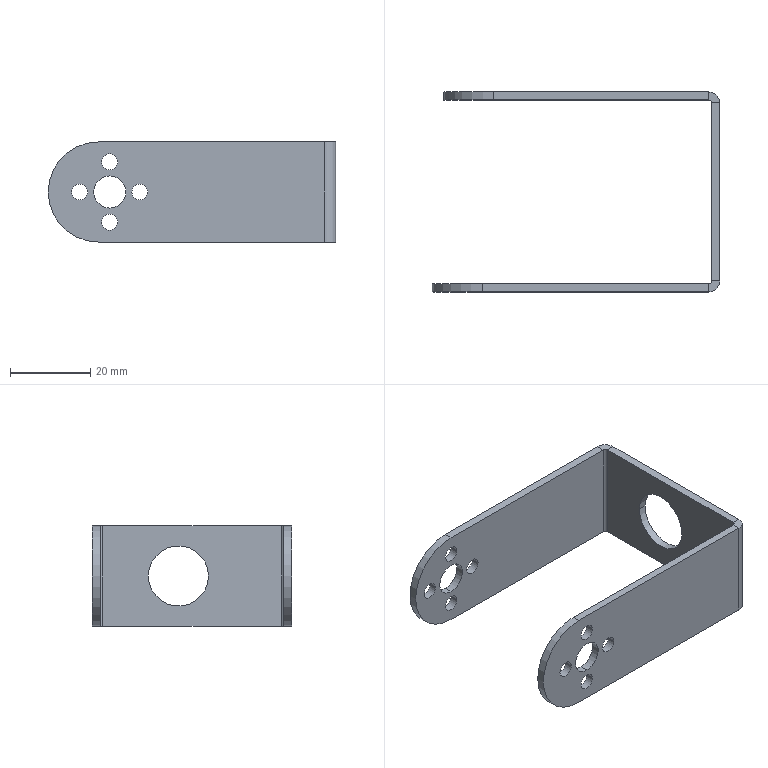Part | SolidWorks | features ICE 3, FlatPattern 1, SM3dBend 1, SMBaseFlange 1, SheetMetal 1 | 1 solid | 44 faces | box 71.712 x 49.895 x 25 mm | volume 8226 mm3 | cylinder 28 | plane 16 | commonest cylinder face diameters 4 x16 8 x4 1.473 x2 5.473 x2 15 x2 25 x2
STEP:
#1=CARTESIAN_POINT('',(-75.172,-2.,-7.5));
#2=VERTEX_POINT('',#1);
#3=CARTESIAN_POINT('',(-79.172,-2.,-7.5));
#4=VERTEX_POINT('',#3);
#5=CARTESIAN_POINT('',(-77.172,-2.,-7.5));
#6=DIRECTION('',(0.,1.,0.));
#7=DIRECTION('',(-1.,0.,0.));
#8=AXIS2_PLACEMENT_3D('',#5,#6,#7);
#9=CIRCLE('',#8,2.);
#10=EDGE_CURVE('',#2,#4,#9,.T.);
#11=ORIENTED_EDGE('',*,*,#10,.F.);
#12=CARTESIAN_POINT('',(-75.172,0.,-7.5));
#13=VERTEX_POINT('',#12);
#14=CARTESIAN_POINT('',(-75.172,-2.,-7.5));
#15=DIRECTION('',(0.,1.,0.));
#16=VECTOR('',#15,1000.);
#17=LINE('',#14,#16);
#18=EDGE_CURVE('',#2,#13,#17,.T.);
#19=ORIENTED_EDGE('',*,*,#18,.T.);
#20=CARTESIAN_POINT('',(-79.172,0.,-7.5));
#21=VERTEX_POINT('',#20);
#22=CARTESIAN_POINT('',(-77.172,0.,-7.5));
#23=DIRECTION('',(0.,1.,0.));
#24=DIRECTION('',(0.,0.,1.));
#25=AXIS2_PLACEMENT_3D('',#22,#23,#24);
#26=CIRCLE('',#25,2.);
#27=EDGE_CURVE('',#13,#21,#26,.T.);
#28=ORIENTED_EDGE('',*,*,#27,.T.);
#29=CARTESIAN_POINT('',(-79.172,-2.,-7.5));
#30=DIRECTION('',(0.,1.,0.));
#31=VECTOR('',#30,1000.);
#32=LINE('',#29,#31);
#33=EDGE_CURVE('',#4,#21,#32,.T.);
#34=ORIENTED_EDGE('',*,*,#33,.F.);
#35=EDGE_LOOP('',(#11,#19,#28,#34));
#36=FACE_OUTER_BOUND('',#35,.T.);
#37=CARTESIAN_POINT('',(-77.172,-2.,-7.5));
#38=DIRECTION('',(0.,1.,0.));
#39=DIRECTION('',(-1.,0.,0.));
#40=AXIS2_PLACEMENT_3D('',#37,#38,#39);
#41=CYLINDRICAL_SURFACE('',#40,2.);
#42=ADVANCED_FACE('',(#36),#41,.F.);
#43=CARTESIAN_POINT('',(-67.672,-2.,0.));
#44=VERTEX_POINT('',#43);
#45=CARTESIAN_POINT('',(-71.672,-2.,0.));
#46=VERTEX_POINT('',#45);
#47=CARTESIAN_POINT('',(-69.672,-2.,0.));
#48=DIRECTION('',(0.,1.,0.));
#49=DIRECTION('',(-1.,0.,0.));
#50=AXIS2_PLACEMENT_3D('',#47,#48,#49);
#51=CIRCLE('',#50,2.);
#52=EDGE_CURVE('',#44,#46,#51,.T.);
#53=ORIENTED_EDGE('',*,*,#52,.F.);
#54=CARTESIAN_POINT('',(-67.672,0.,0.));
#55=VERTEX_POINT('',#54);
#56=CARTESIAN_POINT('',(-67.672,-2.,0.));
#57=DIRECTION('',(0.,1.,0.));
#58=VECTOR('',#57,1000.);
#59=LINE('',#56,#58);
#60=EDGE_CURVE('',#44,#55,#59,.T.);
#61=ORIENTED_EDGE('',*,*,#60,.T.);
#62=CARTESIAN_POINT('',(-71.672,0.,0.));
#63=VERTEX_POINT('',#62);
#64=CARTESIAN_POINT('',(-69.672,0.,0.));
#65=DIRECTION('',(0.,1.,0.));
#66=DIRECTION('',(0.,0.,1.));
#67=AXIS2_PLACEMENT_3D('',#64,#65,#66);
#68=CIRCLE('',#67,2.);
#69=EDGE_CURVE('',#55,#63,#68,.T.);
#70=ORIENTED_EDGE('',*,*,#69,.T.);
#71=CARTESIAN_POINT('',(-71.672,-2.,0.));
#72=DIRECTION('',(0.,1.,0.));
#73=VECTOR('',#72,1000.);
#74=LINE('',#71,#73);
#75=EDGE_CURVE('',#46,#63,#74,.T.);
#76=ORIENTED_EDGE('',*,*,#75,.F.);
#77=EDGE_LOOP('',(#53,#61,#70,#76));
#78=FACE_OUTER_BOUND('',#77,.T.);
#79=CARTESIAN_POINT('',(-69.672,-2.,0.));
#80=DIRECTION('',(0.,1.,0.));
#81=DIRECTION('',(-1.,0.,0.));
#82=AXIS2_PLACEMENT_3D('',#79,#80,#81);
#83=CYLINDRICAL_SURFACE('',#82,2.);
#84=ADVANCED_FACE('',(#78),#83,.F.);
#85=CARTESIAN_POINT('',(-75.172,-2.,7.5));
#86=VERTEX_POINT('',#85);
#87=CARTESIAN_POINT('',(-79.172,-2.,7.5));
#88=VERTEX_POINT('',#87);
#89=CARTESIAN_POINT('',(-77.172,-2.,7.5));
#90=DIRECTION('',(0.,1.,0.));
#91=DIRECTION('',(-1.,0.,0.));
#92=AXIS2_PLACEMENT_3D('',#89,#90,#91);
#93=CIRCLE('',#92,2.);
#94=EDGE_CURVE('',#86,#88,#93,.T.);
#95=ORIENTED_EDGE('',*,*,#94,.F.);
#96=CARTESIAN_POINT('',(-75.172,0.,7.5));
#97=VERTEX_POINT('',#96);
#98=CARTESIAN_POINT('',(-75.172,-2.,7.5));
#99=DIRECTION('',(0.,1.,0.));
#100=VECTOR('',#99,1000.);
#101=LINE('',#98,#100);
#102=EDGE_CURVE('',#86,#97,#101,.T.);
#103=ORIENTED_EDGE('',*,*,#102,.T.);
#104=CARTESIAN_POINT('',(-79.172,0.,7.5));
#105=VERTEX_POINT('',#104);
#106=CARTESIAN_POINT('',(-77.172,0.,7.5));
#107=DIRECTION('',(0.,1.,0.));
#108=DIRECTION('',(0.,0.,1.));
#109=AXIS2_PLACEMENT_3D('',#106,#107,#108);
#110=CIRCLE('',#109,2.);
#111=EDGE_CURVE('',#97,#105,#110,.T.);
#112=ORIENTED_EDGE('',*,*,#111,.T.);
#113=CARTESIAN_POINT('',(-79.172,-2.,7.5));
#114=DIRECTION('',(0.,1.,0.));
#115=VECTOR('',#114,1000.);
#116=LINE('',#113,#115);
#117=EDGE_CURVE('',#88,#105,#116,.T.);
#118=ORIENTED_EDGE('',*,*,#117,.F.);
#119=EDGE_LOOP('',(#95,#103,#112,#118));
#120=FACE_OUTER_BOUND('',#119,.T.);
#121=CARTESIAN_POINT('',(-77.172,-2.,7.5));
#122=DIRECTION('',(0.,1.,0.));
#123=DIRECTION('',(-1.,0.,0.));
#124=AXIS2_PLACEMENT_3D('',#121,#122,#123);
#125=CYLINDRICAL_SURFACE('',#124,2.);
#126=ADVANCED_FACE('',(#120),#125,.F.);
#127=CARTESIAN_POINT('',(-82.672,-2.,0.));
#128=VERTEX_POINT('',#127);
#129=CARTESIAN_POINT('',(-86.672,-2.,0.));
#130=VERTEX_POINT('',#129);
#131=CARTESIAN_POINT('',(-84.672,-2.,0.));
#132=DIRECTION('',(0.,1.,0.));
#133=DIRECTION('',(-1.,0.,0.));
#134=AXIS2_PLACEMENT_3D('',#131,#132,#133);
#135=CIRCLE('',#134,2.);
#136=EDGE_CURVE('',#128,#130,#135,.T.);
#137=ORIENTED_EDGE('',*,*,#136,.F.);
#138=CARTESIAN_POINT('',(-82.672,0.,0.));
#139=VERTEX_POINT('',#138);
#140=CARTESIAN_POINT('',(-82.672,-2.,0.));
#141=DIRECTION('',(0.,1.,0.));
#142=VECTOR('',#141,1000.);
#143=LINE('',#140,#142);
#144=EDGE_CURVE('',#128,#139,#143,.T.);
#145=ORIENTED_EDGE('',*,*,#144,.T.);
#146=CARTESIAN_POINT('',(-86.672,0.,0.));
#147=VERTEX_POINT('',#146);
#148=CARTESIAN_POINT('',(-84.672,0.,0.));
#149=DIRECTION('',(0.,1.,0.));
#150=DIRECTION('',(0.,0.,1.));
#151=AXIS2_PLACEMENT_3D('',#148,#149,#150);
#152=CIRCLE('',#151,2.);
#153=EDGE_CURVE('',#139,#147,#152,.T.);
#154=ORIENTED_EDGE('',*,*,#153,.T.);
#155=CARTESIAN_POINT('',(-86.672,-2.,0.));
#156=DIRECTION('',(0.,1.,0.));
#157=VECTOR('',#156,1000.);
#158=LINE('',#155,#157);
#159=EDGE_CURVE('',#130,#147,#158,.T.);
#160=ORIENTED_EDGE('',*,*,#159,.F.);
#161=EDGE_LOOP('',(#137,#145,#154,#160));
#162=FACE_OUTER_BOUND('',#161,.T.);
#163=CARTESIAN_POINT('',(-84.672,-2.,0.));
#164=DIRECTION('',(0.,1.,0.));
#165=DIRECTION('',(-1.,0.,0.));
#166=AXIS2_PLACEMENT_3D('',#163,#164,#165);
#167=CYLINDRICAL_SURFACE('',#166,2.);
#168=ADVANCED_FACE('',(#162),#167,.F.);
#169=CARTESIAN_POINT('',(-79.172,45.895,-7.5));
#170=VERTEX_POINT('',#169);
#171=CARTESIAN_POINT('',(-75.172,45.895,-7.5));
#172=VERTEX_POINT('',#171);
#173=CARTESIAN_POINT('',(-77.172,45.895,-7.5));
#174=DIRECTION('',(0.,-1.,0.));
#175=DIRECTION('',(1.,0.,0.));
#176=AXIS2_PLACEMENT_3D('',#173,#174,#175);
#177=CIRCLE('',#176,2.);
#178=EDGE_CURVE('',#170,#172,#177,.T.);
#179=ORIENTED_EDGE('',*,*,#178,.T.);
#180=CARTESIAN_POINT('',(-75.172,47.895,-7.5));
#181=VERTEX_POINT('',#180);
#182=CARTESIAN_POINT('',(-75.172,-2.,-7.5));
#183=DIRECTION('',(0.,1.,0.));
#184=VECTOR('',#183,1000.);
#185=LINE('',#182,#184);
#186=EDGE_CURVE('',#172,#181,#185,.T.);
#187=ORIENTED_EDGE('',*,*,#186,.T.);
#188=CARTESIAN_POINT('',(-79.172,47.895,-7.5));
#189=VERTEX_POINT('',#188);
#190=CARTESIAN_POINT('',(-77.172,47.895,-7.5));
#191=DIRECTION('',(0.,-1.,0.));
#192=DIRECTION('',(1.,0.,0.));
#193=AXIS2_PLACEMENT_3D('',#190,#191,#192);
#194=CIRCLE('',#193,2.);
#195=EDGE_CURVE('',#189,#181,#194,.T.);
#196=ORIENTED_EDGE('',*,*,#195,.F.);
#197=CARTESIAN_POINT('',(-79.172,-2.,-7.5));
#198=DIRECTION('',(0.,1.,0.));
#199=VECTOR('',#198,1000.);
#200=LINE('',#197,#199);
#201=EDGE_CURVE('',#170,#189,#200,.T.);
#202=ORIENTED_EDGE('',*,*,#201,.F.);
#203=EDGE_LOOP('',(#179,#187,#196,#202));
#204=FACE_OUTER_BOUND('',#203,.T.);
#205=CARTESIAN_POINT('',(-77.172,-2.,-7.5));
#206=DIRECTION('',(0.,1.,0.));
#207=DIRECTION('',(-1.,0.,0.));
#208=AXIS2_PLACEMENT_3D('',#205,#206,#207);
#209=CYLINDRICAL_SURFACE('',#208,2.);
#210=ADVANCED_FACE('',(#204),#209,.F.);
#211=CARTESIAN_POINT('',(-71.672,45.895,0.));
#212=VERTEX_POINT('',#211);
#213=CARTESIAN_POINT('',(-67.672,45.895,0.));
#214=VERTEX_POINT('',#213);
#215=CARTESIAN_POINT('',(-69.672,45.895,0.));
#216=DIRECTION('',(0.,-1.,0.));
#217=DIRECTION('',(1.,0.,0.));
#218=AXIS2_PLACEMENT_3D('',#215,#216,#217);
#219=CIRCLE('',#218,2.);
#220=EDGE_CURVE('',#212,#214,#219,.T.);
#221=ORIENTED_EDGE('',*,*,#220,.T.);
#222=CARTESIAN_POINT('',(-67.672,47.895,0.));
#223=VERTEX_POINT('',#222);
#224=CARTESIAN_POINT('',(-67.672,-2.,0.));
#225=DIRECTION('',(0.,1.,0.));
#226=VECTOR('',#225,1000.);
#227=LINE('',#224,#226);
#228=EDGE_CURVE('',#214,#223,#227,.T.);
#229=ORIENTED_EDGE('',*,*,#228,.T.);
#230=CARTESIAN_POINT('',(-71.672,47.895,0.));
#231=VERTEX_POINT('',#230);
#232=CARTESIAN_POINT('',(-69.672,47.895,0.));
#233=DIRECTION('',(0.,-1.,0.));
#234=DIRECTION('',(1.,0.,0.));
#235=AXIS2_PLACEMENT_3D('',#232,#233,#234);
#236=CIRCLE('',#235,2.);
#237=EDGE_CURVE('',#231,#223,#236,.T.);
#238=ORIENTED_EDGE('',*,*,#237,.F.);
#239=CARTESIAN_POINT('',(-71.672,-2.,0.));
#240=DIRECTION('',(0.,1.,0.));
#241=VECTOR('',#240,1000.);
#242=LINE('',#239,#241);
#243=EDGE_CURVE('',#212,#231,#242,.T.);
#244=ORIENTED_EDGE('',*,*,#243,.F.);
#245=EDGE_LOOP('',(#221,#229,#238,#244));
#246=FACE_OUTER_BOUND('',#245,.T.);
#247=CARTESIAN_POINT('',(-69.672,-2.,0.));
#248=DIRECTION('',(0.,1.,0.));
#249=DIRECTION('',(-1.,0.,0.));
#250=AXIS2_PLACEMENT_3D('',#247,#248,#249);
#251=CYLINDRICAL_SURFACE('',#250,2.);
#252=ADVANCED_FACE('',(#246),#251,.F.);
#253=CARTESIAN_POINT('',(-79.172,45.895,7.5));
#254=VERTEX_POINT('',#253);
#255=CARTESIAN_POINT('',(-75.172,45.895,7.5));
#256=VERTEX_POINT('',#255);
#257=CARTESIAN_POINT('',(-77.172,45.895,7.5));
#258=DIRECTION('',(0.,-1.,0.));
#259=DIRECTION('',(1.,0.,0.));
#260=AXIS2_PLACEMENT_3D('',#257,#258,#259);
#261=CIRCLE('',#260,2.);
#262=EDGE_CURVE('',#254,#256,#261,.T.);
#263=ORIENTED_EDGE('',*,*,#262,.T.);
#264=CARTESIAN_POINT('',(-75.172,47.895,7.5));
#265=VERTEX_POINT('',#264);
#266=CARTESIAN_POINT('',(-75.172,-2.,7.5));
#267=DIRECTION('',(0.,1.,0.));
#268=VECTOR('',#267,1000.);
#269=LINE('',#266,#268);
#270=EDGE_CURVE('',#256,#265,#269,.T.);
#271=ORIENTED_EDGE('',*,*,#270,.T.);
#272=CARTESIAN_POINT('',(-79.172,47.895,7.5));
#273=VERTEX_POINT('',#272);
#274=CARTESIAN_POINT('',(-77.172,47.895,7.5));
#275=DIRECTION('',(0.,-1.,0.));
#276=DIRECTION('',(1.,0.,0.));
#277=AXIS2_PLACEMENT_3D('',#274,#275,#276);
#278=CIRCLE('',#277,2.);
#279=EDGE_CURVE('',#273,#265,#278,.T.);
#280=ORIENTED_EDGE('',*,*,#279,.F.);
#281=CARTESIAN_POINT('',(-79.172,-2.,7.5));
#282=DIRECTION('',(0.,1.,0.));
#283=VECTOR('',#282,1000.);
#284=LINE('',#281,#283);
#285=EDGE_CURVE('',#254,#273,#284,.T.);
#286=ORIENTED_EDGE('',*,*,#285,.F.);
#287=EDGE_LOOP('',(#263,#271,#280,#286));
#288=FACE_OUTER_BOUND('',#287,.T.);
#289=CARTESIAN_POINT('',(-77.172,-2.,7.5));
#290=DIRECTION('',(0.,1.,0.));
#291=DIRECTION('',(-1.,0.,0.));
#292=AXIS2_PLACEMENT_3D('',#289,#290,#291);
#293=CYLINDRICAL_SURFACE('',#292,2.);
#294=ADVANCED_FACE('',(#288),#293,.F.);
#295=CARTESIAN_POINT('',(-86.672,45.895,0.));
#296=VERTEX_POINT('',#295);
#297=CARTESIAN_POINT('',(-82.672,45.895,0.));
#298=VERTEX_POINT('',#297);
#299=CARTESIAN_POINT('',(-84.672,45.895,0.));
#300=DIRECTION('',(0.,-1.,0.));
#301=DIRECTION('',(1.,0.,0.));
#302=AXIS2_PLACEMENT_3D('',#299,#300,#301);
#303=CIRCLE('',#302,2.);
#304=EDGE_CURVE('',#296,#298,#303,.T.);
#305=ORIENTED_EDGE('',*,*,#304,.T.);
#306=CARTESIAN_POINT('',(-82.672,47.895,0.));
#307=VERTEX_POINT('',#306);
#308=CARTESIAN_POINT('',(-82.672,-2.,0.));
#309=DIRECTION('',(0.,1.,0.));
#310=VECTOR('',#309,1000.);
#311=LINE('',#308,#310);
#312=EDGE_CURVE('',#298,#307,#311,.T.);
#313=ORIENTED_EDGE('',*,*,#312,.T.);
#314=CARTESIAN_POINT('',(-86.672,47.895,0.));
#315=VERTEX_POINT('',#314);
#316=CARTESIAN_POINT('',(-84.672,47.895,0.));
#317=DIRECTION('',(0.,-1.,0.));
#318=DIRECTION('',(1.,0.,0.));
#319=AXIS2_PLACEMENT_3D('',#316,#317,#318);
#320=CIRCLE('',#319,2.);
#321=EDGE_CURVE('',#315,#307,#320,.T.);
#322=ORIENTED_EDGE('',*,*,#321,.F.);
#323=CARTESIAN_POINT('',(-86.672,-2.,0.));
#324=DIRECTION('',(0.,1.,0.));
#325=VECTOR('',#324,1000.);
#326=LINE('',#323,#325);
#327=EDGE_CURVE('',#296,#315,#326,.T.);
#328=ORIENTED_EDGE('',*,*,#327,.F.);
#329=EDGE_LOOP('',(#305,#313,#322,#328));
#330=FACE_OUTER_BOUND('',#329,.T.);
#331=CARTESIAN_POINT('',(-84.672,-2.,0.));
#332=DIRECTION('',(0.,1.,0.));
#333=DIRECTION('',(-1.,0.,0.));
#334=AXIS2_PLACEMENT_3D('',#331,#332,#333);
#335=CYLINDRICAL_SURFACE('',#334,2.);
#336=ADVANCED_FACE('',(#330),#335,.F.);
#337=CARTESIAN_POINT('',(-22.788,33.833,0.));
#338=VERTEX_POINT('',#337);
#339=CARTESIAN_POINT('',(-22.788,18.833,0.));
#340=VERTEX_POINT('',#339);
#341=CARTESIAN_POINT('',(-22.788,26.333,0.));
#342=DIRECTION('',(-1.,0.,0.));
#343=DIRECTION('',(0.,-1.,0.));
#344=AXIS2_PLACEMENT_3D('',#341,#342,#343);
#345=CIRCLE('',#344,7.5);
#346=EDGE_CURVE('',#338,#340,#345,.T.);
#347=ORIENTED_EDGE('',*,*,#346,.T.);
#348=CARTESIAN_POINT('',(-20.788,18.833,0.));
#349=VERTEX_POINT('',#348);
#350=CARTESIAN_POINT('',(-30.788,18.833,0.));
#351=DIRECTION('',(1.,0.,0.));
#352=VECTOR('',#351,1000.);
#353=LINE('',#350,#352);
#354=EDGE_CURVE('',#340,#349,#353,.T.);
#355=ORIENTED_EDGE('',*,*,#354,.T.);
#356=CARTESIAN_POINT('',(-20.788,33.833,0.));
#357=VERTEX_POINT('',#356);
#358=CARTESIAN_POINT('',(-20.788,26.333,0.));
#359=DIRECTION('',(1.,0.,0.));
#360=DIRECTION('',(0.,1.,0.));
#361=AXIS2_PLACEMENT_3D('',#358,#359,#360);
#362=CIRCLE('',#361,7.5);
#363=EDGE_CURVE('',#349,#357,#362,.T.);
#364=ORIENTED_EDGE('',*,*,#363,.T.);
#365=CARTESIAN_POINT('',(-30.788,33.833,0.));
#366=DIRECTION('',(1.,0.,0.));
#367=VECTOR('',#366,1000.);
#368=LINE('',#365,#367);
#369=EDGE_CURVE('',#338,#357,#368,.T.);
#370=ORIENTED_EDGE('',*,*,#369,.F.);
#371=EDGE_LOOP('',(#347,#355,#364,#370));
#372=FACE_OUTER_BOUND('',#371,.T.);
#373=CARTESIAN_POINT('',(-30.788,26.333,0.));
#374=DIRECTION('',(1.,0.,0.));
#375=DIRECTION('',(0.,1.,0.));
#376=AXIS2_PLACEMENT_3D('',#373,#374,#375);
#377=CYLINDRICAL_SURFACE('',#376,7.5);
#378=ADVANCED_FACE('',(#372),#377,.F.);
#379=CARTESIAN_POINT('',(-77.172,-2.,-4.));
#380=VERTEX_POINT('',#379);
#381=CARTESIAN_POINT('',(-77.172,-2.,4.));
#382=VERTEX_POINT('',#381);
#383=CARTESIAN_POINT('',(-77.172,-2.,0.));
#384=DIRECTION('',(0.,1.,0.));
#385=DIRECTION('',(0.,0.,1.));
#386=AXIS2_PLACEMENT_3D('',#383,#384,#385);
#387=CIRCLE('',#386,4.);
#388=EDGE_CURVE('',#380,#382,#387,.T.);
#389=ORIENTED_EDGE('',*,*,#388,.F.);
#390=CARTESIAN_POINT('',(-77.172,0.,-4.));
#391=VERTEX_POINT('',#390);
#392=CARTESIAN_POINT('',(-77.172,-2.,-4.));
#393=DIRECTION('',(0.,1.,0.));
#394=VECTOR('',#393,1000.);
#395=LINE('',#392,#394);
#396=EDGE_CURVE('',#380,#391,#395,.T.);
#397=ORIENTED_EDGE('',*,*,#396,.T.);
#398=CARTESIAN_POINT('',(-77.172,0.,4.));
#399=VERTEX_POINT('',#398);
#400=CARTESIAN_POINT('',(-77.172,0.,0.));
#401=DIRECTION('',(0.,1.,0.));
#402=DIRECTION('',(0.,0.,1.));
#403=AXIS2_PLACEMENT_3D('',#400,#401,#402);
#404=CIRCLE('',#403,4.);
#405=EDGE_CURVE('',#391,#399,#404,.T.);
#406=ORIENTED_EDGE('',*,*,#405,.T.);
#407=CARTESIAN_POINT('',(-77.172,-2.,4.));
#408=DIRECTION('',(0.,1.,0.));
#409=VECTOR('',#408,1000.);
#410=LINE('',#407,#409);
#411=EDGE_CURVE('',#382,#399,#410,.T.);
#412=ORIENTED_EDGE('',*,*,#411,.F.);
#413=EDGE_LOOP('',(#389,#397,#406,#412));
#414=FACE_OUTER_BOUND('',#413,.T.);
#415=CARTESIAN_POINT('',(-77.172,-2.,0.));
#416=DIRECTION('',(0.,1.,0.));
#417=DIRECTION('',(0.,0.,1.));
#418=AXIS2_PLACEMENT_3D('',#415,#416,#417);
#419=CYLINDRICAL_SURFACE('',#418,4.);
#420=ADVANCED_FACE('',(#414),#419,.F.);
#421=CARTESIAN_POINT('',(-77.172,45.895,4.));
#422=VERTEX_POINT('',#421);
#423=CARTESIAN_POINT('',(-77.172,45.895,-4.));
#424=VERTEX_POINT('',#423);
#425=CARTESIAN_POINT('',(-77.172,45.895,0.));
#426=DIRECTION('',(0.,-1.,0.));
#427=DIRECTION('',(1.,0.,0.));
#428=AXIS2_PLACEMENT_3D('',#425,#426,#427);
#429=CIRCLE('',#428,4.);
#430=EDGE_CURVE('',#422,#424,#429,.T.);
#431=ORIENTED_EDGE('',*,*,#430,.T.);
#432=CARTESIAN_POINT('',(-77.172,47.895,-4.));
#433=VERTEX_POINT('',#432);
#434=CARTESIAN_POINT('',(-77.172,-2.,-4.));
#435=DIRECTION('',(0.,1.,0.));
#436=VECTOR('',#435,1000.);
#437=LINE('',#434,#436);
#438=EDGE_CURVE('',#424,#433,#437,.T.);
#439=ORIENTED_EDGE('',*,*,#438,.T.);
#440=CARTESIAN_POINT('',(-77.172,47.895,4.));
#441=VERTEX_POINT('',#440);
#442=CARTESIAN_POINT('',(-77.172,47.895,0.));
#443=DIRECTION('',(0.,1.,0.));
#444=DIRECTION('',(0.,0.,1.));
#445=AXIS2_PLACEMENT_3D('',#442,#443,#444);
#446=CIRCLE('',#445,4.);
#447=EDGE_CURVE('',#433,#441,#446,.T.);
#448=ORIENTED_EDGE('',*,*,#447,.T.);
#449=CARTESIAN_POINT('',(-77.172,-2.,4.));
#450=DIRECTION('',(0.,1.,0.));
#451=VECTOR('',#450,1000.);
#452=LINE('',#449,#451);
#453=EDGE_CURVE('',#422,#441,#452,.T.);
#454=ORIENTED_EDGE('',*,*,#453,.F.);
#455=EDGE_LOOP('',(#431,#439,#448,#454));
#456=FACE_OUTER_BOUND('',#455,.T.);
#457=CARTESIAN_POINT('',(-77.172,-2.,0.));
#458=DIRECTION('',(0.,1.,0.));
#459=DIRECTION('',(0.,0.,1.));
#460=AXIS2_PLACEMENT_3D('',#457,#458,#459);
#461=CYLINDRICAL_SURFACE('',#460,4.);
#462=ADVANCED_FACE('',(#456),#461,.F.);
#463=ORIENTED_EDGE('',*,*,#346,.F.);
#464=CARTESIAN_POINT('',(-22.788,26.333,0.));
#465=DIRECTION('',(-1.,0.,0.));
#466=DIRECTION('',(0.,-1.,0.));
#467=AXIS2_PLACEMENT_3D('',#464,#465,#466);
#468=CIRCLE('',#467,7.5);
#469=EDGE_CURVE('',#340,#338,#468,.T.);
#470=ORIENTED_EDGE('',*,*,#469,.F.);
#471=EDGE_LOOP('',(#463,#470));
#472=FACE_BOUND('',#471,.T.);
#473=CARTESIAN_POINT('',(-22.788,0.7366,12.5));
#474=VERTEX_POINT('',#473);
#475=CARTESIAN_POINT('',(-22.788,45.159,12.5));
#476=VERTEX_POINT('',#475);
#477=CARTESIAN_POINT('',(-22.788,-58.466,12.5));
#478=DIRECTION('',(0.,1.,0.));
#479=VECTOR('',#478,1000.);
#480=LINE('',#477,#479);
#481=EDGE_CURVE('',#474,#476,#480,.T.);
#482=ORIENTED_EDGE('',*,*,#481,.T.);
#483=CARTESIAN_POINT('',(-22.788,45.159,-12.5));
#484=VERTEX_POINT('',#483);
#485=CARTESIAN_POINT('',(-22.788,45.159,0.));
#486=DIRECTION('',(0.,0.,-1.));
#487=VECTOR('',#486,1000.);
#488=LINE('',#485,#487);
#489=EDGE_CURVE('',#476,#484,#488,.T.);
#490=ORIENTED_EDGE('',*,*,#489,.T.);
#491=CARTESIAN_POINT('',(-22.788,0.7366,-12.5));
#492=VERTEX_POINT('',#491);
#493=CARTESIAN_POINT('',(-22.788,-58.466,-12.5));
#494=DIRECTION('',(0.,-1.,0.));
#495=VECTOR('',#494,1000.);
#496=LINE('',#493,#495);
#497=EDGE_CURVE('',#484,#492,#496,.T.);
#498=ORIENTED_EDGE('',*,*,#497,.T.);
#499=CARTESIAN_POINT('',(-22.788,0.7366,0.));
#500=DIRECTION('',(0.,0.,-1.));
#501=VECTOR('',#500,1000.);
#502=LINE('',#499,#501);
#503=EDGE_CURVE('',#474,#492,#502,.T.);
#504=ORIENTED_EDGE('',*,*,#503,.F.);
#505=EDGE_LOOP('',(#482,#490,#498,#504));
#506=FACE_OUTER_BOUND('',#505,.T.);
#507=CARTESIAN_POINT('',(-22.788,-58.466,0.));
#508=DIRECTION('',(-1.,0.,0.));
#509=DIRECTION('',(0.,0.,1.));
#510=AXIS2_PLACEMENT_3D('',#507,#508,#509);
#511=PLANE('',#510);
#512=ADVANCED_FACE('',(#472,#506),#511,.T.);
#513=CARTESIAN_POINT('',(-20.788,0.7366,12.5));
#514=VERTEX_POINT('',#513);
#515=CARTESIAN_POINT('',(-20.788,45.159,12.5));
#516=VERTEX_POINT('',#515);
#517=CARTESIAN_POINT('',(-20.788,-58.466,12.5));
#518=DIRECTION('',(0.,1.,0.));
#519=VECTOR('',#518,1000.);
#520=LINE('',#517,#519);
#521=EDGE_CURVE('',#514,#516,#520,.T.);
#522=ORIENTED_EDGE('',*,*,#521,.T.);
#523=CARTESIAN_POINT('',(-20.788,45.159,12.5));
#524=DIRECTION('',(-1.,0.,0.));
#525=VECTOR('',#524,1000.);
#526=LINE('',#523,#525);
#527=EDGE_CURVE('',#516,#476,#526,.T.);
#528=ORIENTED_EDGE('',*,*,#527,.T.);
#529=ORIENTED_EDGE('',*,*,#481,.F.);
#530=CARTESIAN_POINT('',(-20.788,0.7366,12.5));
#531=DIRECTION('',(-1.,0.,0.));
#532=VECTOR('',#531,1000.);
#533=LINE('',#530,#532);
#534=EDGE_CURVE('',#514,#474,#533,.T.);
#535=ORIENTED_EDGE('',*,*,#534,.F.);
#536=EDGE_LOOP('',(#522,#528,#529,#535));
#537=FACE_OUTER_BOUND('',#536,.T.);
#538=CARTESIAN_POINT('',(-20.788,-58.466,12.5));
#539=DIRECTION('',(0.,0.,1.));
#540=DIRECTION('',(0.,1.,0.));
#541=AXIS2_PLACEMENT_3D('',#538,#539,#540);
#542=PLANE('',#541);
#543=ADVANCED_FACE('',(#537),#542,.T.);
#544=ORIENTED_EDGE('',*,*,#497,.F.);
#545=CARTESIAN_POINT('',(-20.788,45.159,-12.5));
#546=VERTEX_POINT('',#545);
#547=CARTESIAN_POINT('',(-20.788,45.159,-12.5));
#548=DIRECTION('',(1.,0.,0.));
#549=VECTOR('',#548,1000.);
#550=LINE('',#547,#549);
#551=EDGE_CURVE('',#484,#546,#550,.T.);
#552=ORIENTED_EDGE('',*,*,#551,.T.);
#553=CARTESIAN_POINT('',(-20.788,0.7366,-12.5));
#554=VERTEX_POINT('',#553);
#555=CARTESIAN_POINT('',(-20.788,-58.466,-12.5));
#556=DIRECTION('',(0.,-1.,0.));
#557=VECTOR('',#556,1000.);
#558=LINE('',#555,#557);
#559=EDGE_CURVE('',#546,#554,#558,.T.);
#560=ORIENTED_EDGE('',*,*,#559,.T.);
#561=CARTESIAN_POINT('',(-20.788,0.7366,-12.5));
#562=DIRECTION('',(1.,0.,0.));
#563=VECTOR('',#562,1000.);
#564=LINE('',#561,#563);
#565=EDGE_CURVE('',#492,#554,#564,.T.);
#566=ORIENTED_EDGE('',*,*,#565,.F.);
#567=EDGE_LOOP('',(#544,#552,#560,#566));
#568=FACE_OUTER_BOUND('',#567,.T.);
#569=CARTESIAN_POINT('',(-20.788,-58.466,-12.5));
#570=DIRECTION('',(0.,0.,-1.));
#571=DIRECTION('',(0.,-1.,0.));
#572=AXIS2_PLACEMENT_3D('',#569,#570,#571);
#573=PLANE('',#572);
#574=ADVANCED_FACE('',(#568),#573,.T.);
#575=CARTESIAN_POINT('',(-20.788,26.333,0.));
#576=DIRECTION('',(1.,0.,0.));
#577=DIRECTION('',(0.,1.,0.));
#578=AXIS2_PLACEMENT_3D('',#575,#576,#577);
#579=CIRCLE('',#578,7.5);
#580=EDGE_CURVE('',#357,#349,#579,.T.);
#581=ORIENTED_EDGE('',*,*,#580,.F.);
#582=ORIENTED_EDGE('',*,*,#363,.F.);
#583=EDGE_LOOP('',(#581,#582));
#584=FACE_BOUND('',#583,.T.);
#585=CARTESIAN_POINT('',(-20.788,45.159,0.));
#586=DIRECTION('',(0.,0.,-1.));
#587=VECTOR('',#586,1000.);
#588=LINE('',#585,#587);
#589=EDGE_CURVE('',#516,#546,#588,.T.);
#590=ORIENTED_EDGE('',*,*,#589,.F.);
#591=ORIENTED_EDGE('',*,*,#521,.F.);
#592=CARTESIAN_POINT('',(-20.788,0.7366,0.));
#593=DIRECTION('',(0.,0.,-1.));
#594=VECTOR('',#593,1000.);
#595=LINE('',#592,#594);
#596=EDGE_CURVE('',#514,#554,#595,.T.);
#597=ORIENTED_EDGE('',*,*,#596,.T.);
#598=ORIENTED_EDGE('',*,*,#559,.F.);
#599=EDGE_LOOP('',(#590,#591,#597,#598));
#600=FACE_OUTER_BOUND('',#599,.T.);
#601=CARTESIAN_POINT('',(-20.788,-58.466,0.));
#602=DIRECTION('',(-1.,0.,0.));
#603=DIRECTION('',(0.,0.,1.));
#604=AXIS2_PLACEMENT_3D('',#601,#602,#603);
#605=PLANE('',#604);
#606=ADVANCED_FACE('',(#584,#600),#605,.F.);
#607=CARTESIAN_POINT('',(-80.,0.,-12.5));
#608=VERTEX_POINT('',#607);
#609=CARTESIAN_POINT('',(-80.,0.,12.5));
#610=VERTEX_POINT('',#609);
#611=CARTESIAN_POINT('',(-80.,0.,0.));
#612=DIRECTION('',(0.,1.,0.));
#613=DIRECTION('',(0.,0.,1.));
#614=AXIS2_PLACEMENT_3D('',#611,#612,#613);
#615=CIRCLE('',#614,12.5);
#616=EDGE_CURVE('',#608,#610,#615,.T.);
#617=ORIENTED_EDGE('',*,*,#616,.F.);
#618=CARTESIAN_POINT('',(-80.,-2.,-12.5));
#619=VERTEX_POINT('',#618);
#620=CARTESIAN_POINT('',(-80.,-2.,-12.5));
#621=DIRECTION('',(0.,1.,0.));
#622=VECTOR('',#621,1000.);
#623=LINE('',#620,#622);
#624=EDGE_CURVE('',#619,#608,#623,.T.);
#625=ORIENTED_EDGE('',*,*,#624,.F.);
#626=CARTESIAN_POINT('',(-80.,-2.,12.5));
#627=VERTEX_POINT('',#626);
#628=CARTESIAN_POINT('',(-80.,-2.,0.));
#629=DIRECTION('',(0.,1.,0.));
#630=DIRECTION('',(0.,0.,1.));
#631=AXIS2_PLACEMENT_3D('',#628,#629,#630);
#632=CIRCLE('',#631,12.5);
#633=EDGE_CURVE('',#619,#627,#632,.T.);
#634=ORIENTED_EDGE('',*,*,#633,.T.);
#635=CARTESIAN_POINT('',(-80.,-2.,12.5));
#636=DIRECTION('',(0.,1.,0.));
#637=VECTOR('',#636,1000.);
#638=LINE('',#635,#637);
#639=EDGE_CURVE('',#627,#610,#638,.T.);
#640=ORIENTED_EDGE('',*,*,#639,.T.);
#641=EDGE_LOOP('',(#617,#625,#634,#640));
#642=FACE_OUTER_BOUND('',#641,.T.);
#643=CARTESIAN_POINT('',(-80.,-2.,0.));
#644=DIRECTION('',(0.,1.,0.));
#645=DIRECTION('',(0.,0.,1.));
#646=AXIS2_PLACEMENT_3D('',#643,#644,#645);
#647=CYLINDRICAL_SURFACE('',#646,12.5);
#648=ADVANCED_FACE('',(#642),#647,.T.);
#649=CARTESIAN_POINT('',(-77.172,-2.,-7.5));
#650=DIRECTION('',(0.,1.,0.));
#651=DIRECTION('',(-1.,0.,0.));
#652=AXIS2_PLACEMENT_3D('',#649,#650,#651);
#653=CIRCLE('',#652,2.);
#654=EDGE_CURVE('',#4,#2,#653,.T.);
#655=ORIENTED_EDGE('',*,*,#654,.T.);
#656=ORIENTED_EDGE('',*,*,#10,.T.);
#657=EDGE_LOOP('',(#655,#656));
#658=FACE_BOUND('',#657,.T.);
#659=CARTESIAN_POINT('',(-69.672,-2.,0.));
#660=DIRECTION('',(0.,1.,0.));
#661=DIRECTION('',(-1.,0.,0.));
#662=AXIS2_PLACEMENT_3D('',#659,#660,#661);
#663=CIRCLE('',#662,2.);
#664=EDGE_CURVE('',#46,#44,#663,.T.);
#665=ORIENTED_EDGE('',*,*,#664,.T.);
#666=ORIENTED_EDGE('',*,*,#52,.T.);
#667=EDGE_LOOP('',(#665,#666));
#668=FACE_BOUND('',#667,.T.);
#669=CARTESIAN_POINT('',(-77.172,-2.,7.5));
#670=DIRECTION('',(0.,1.,0.));
#671=DIRECTION('',(-1.,0.,0.));
#672=AXIS2_PLACEMENT_3D('',#669,#670,#671);
#673=CIRCLE('',#672,2.);
#674=EDGE_CURVE('',#88,#86,#673,.T.);
#675=ORIENTED_EDGE('',*,*,#674,.T.);
#676=ORIENTED_EDGE('',*,*,#94,.T.);
#677=EDGE_LOOP('',(#675,#676));
#678=FACE_BOUND('',#677,.T.);
#679=CARTESIAN_POINT('',(-84.672,-2.,0.));
#680=DIRECTION('',(0.,1.,0.));
#681=DIRECTION('',(-1.,0.,0.));
#682=AXIS2_PLACEMENT_3D('',#679,#680,#681);
#683=CIRCLE('',#682,2.);
#684=EDGE_CURVE('',#130,#128,#683,.T.);
#685=ORIENTED_EDGE('',*,*,#684,.T.);
#686=ORIENTED_EDGE('',*,*,#136,.T.);
#687=EDGE_LOOP('',(#685,#686));
#688=FACE_BOUND('',#687,.T.);
#689=CARTESIAN_POINT('',(-77.172,-2.,0.));
#690=DIRECTION('',(0.,1.,0.));
#691=DIRECTION('',(0.,0.,1.));
#692=AXIS2_PLACEMENT_3D('',#689,#690,#691);
#693=CIRCLE('',#692,4.);
#694=EDGE_CURVE('',#382,#380,#693,.T.);
#695=ORIENTED_EDGE('',*,*,#694,.T.);
#696=ORIENTED_EDGE('',*,*,#388,.T.);
#697=EDGE_LOOP('',(#695,#696));
#698=FACE_BOUND('',#697,.T.);
#699=CARTESIAN_POINT('',(-23.525,-2.,12.5));
#700=VERTEX_POINT('',#699);
#701=CARTESIAN_POINT('',(-23.525,-2.,-12.5));
#702=VERTEX_POINT('',#701);
#703=CARTESIAN_POINT('',(-23.525,-2.,0.));
#704=DIRECTION('',(0.,0.,-1.));
#705=VECTOR('',#704,1000.);
#706=LINE('',#703,#705);
#707=EDGE_CURVE('',#700,#702,#706,.T.);
#708=ORIENTED_EDGE('',*,*,#707,.F.);
#709=CARTESIAN_POINT('',(-80.,-2.,12.5));
#710=DIRECTION('',(1.,0.,0.));
#711=VECTOR('',#710,1000.);
#712=LINE('',#709,#711);
#713=EDGE_CURVE('',#627,#700,#712,.T.);
#714=ORIENTED_EDGE('',*,*,#713,.F.);
#715=ORIENTED_EDGE('',*,*,#633,.F.);
#716=CARTESIAN_POINT('',(-80.,-2.,-12.5));
#717=DIRECTION('',(-1.,0.,0.));
#718=VECTOR('',#717,1000.);
#719=LINE('',#716,#718);
#720=EDGE_CURVE('',#702,#619,#719,.T.);
#721=ORIENTED_EDGE('',*,*,#720,.F.);
#722=EDGE_LOOP('',(#708,#714,#715,#721));
#723=FACE_OUTER_BOUND('',#722,.T.);
#724=CARTESIAN_POINT('',(-80.,-2.,0.));
#725=DIRECTION('',(0.,1.,0.));
#726=DIRECTION('',(0.,0.,1.));
#727=AXIS2_PLACEMENT_3D('',#724,#725,#726);
#728=PLANE('',#727);
#729=ADVANCED_FACE('',(#658,#668,#678,#688,#698,#723),#728,.F.);
#730=ORIENTED_EDGE('',*,*,#713,.T.);
#731=CARTESIAN_POINT('',(-23.525,0.,12.5));
#732=VERTEX_POINT('',#731);
#733=CARTESIAN_POINT('',(-23.525,-2.,12.5));
#734=DIRECTION('',(0.,1.,0.));
#735=VECTOR('',#734,1000.);
#736=LINE('',#733,#735);
#737=EDGE_CURVE('',#700,#732,#736,.T.);
#738=ORIENTED_EDGE('',*,*,#737,.T.);
#739=CARTESIAN_POINT('',(-80.,0.,12.5));
#740=DIRECTION('',(1.,0.,0.));
#741=VECTOR('',#740,1000.);
#742=LINE('',#739,#741);
#743=EDGE_CURVE('',#610,#732,#742,.T.);
#744=ORIENTED_EDGE('',*,*,#743,.F.);
#745=ORIENTED_EDGE('',*,*,#639,.F.);
#746=EDGE_LOOP('',(#730,#738,#744,#745));
#747=FACE_OUTER_BOUND('',#746,.T.);
#748=CARTESIAN_POINT('',(-80.,-2.,12.5));
#749=DIRECTION('',(0.,0.,1.));
#750=DIRECTION('',(1.,0.,0.));
#751=AXIS2_PLACEMENT_3D('',#748,#749,#750);
#752=PLANE('',#751);
#753=ADVANCED_FACE('',(#747),#752,.T.);
#754=CARTESIAN_POINT('',(-77.172,0.,-7.5));
#755=DIRECTION('',(0.,1.,0.));
#756=DIRECTION('',(0.,0.,1.));
#757=AXIS2_PLACEMENT_3D('',#754,#755,#756);
#758=CIRCLE('',#757,2.);
#759=EDGE_CURVE('',#21,#13,#758,.T.);
#760=ORIENTED_EDGE('',*,*,#759,.F.);
#761=ORIENTED_EDGE('',*,*,#27,.F.);
#762=EDGE_LOOP('',(#760,#761));
#763=FACE_BOUND('',#762,.T.);
#764=CARTESIAN_POINT('',(-69.672,0.,0.));
#765=DIRECTION('',(0.,1.,0.));
#766=DIRECTION('',(0.,0.,1.));
#767=AXIS2_PLACEMENT_3D('',#764,#765,#766);
#768=CIRCLE('',#767,2.);
#769=EDGE_CURVE('',#63,#55,#768,.T.);
#770=ORIENTED_EDGE('',*,*,#769,.F.);
#771=ORIENTED_EDGE('',*,*,#69,.F.);
#772=EDGE_LOOP('',(#770,#771));
#773=FACE_BOUND('',#772,.T.);
#774=CARTESIAN_POINT('',(-77.172,0.,7.5));
#775=DIRECTION('',(0.,1.,0.));
#776=DIRECTION('',(0.,0.,1.));
#777=AXIS2_PLACEMENT_3D('',#774,#775,#776);
#778=CIRCLE('',#777,2.);
#779=EDGE_CURVE('',#105,#97,#778,.T.);
#780=ORIENTED_EDGE('',*,*,#779,.F.);
#781=ORIENTED_EDGE('',*,*,#111,.F.);
#782=EDGE_LOOP('',(#780,#781));
#783=FACE_BOUND('',#782,.T.);
#784=CARTESIAN_POINT('',(-84.672,0.,0.));
#785=DIRECTION('',(0.,1.,0.));
#786=DIRECTION('',(0.,0.,1.));
#787=AXIS2_PLACEMENT_3D('',#784,#785,#786);
#788=CIRCLE('',#787,2.);
#789=EDGE_CURVE('',#147,#139,#788,.T.);
#790=ORIENTED_EDGE('',*,*,#789,.F.);
#791=ORIENTED_EDGE('',*,*,#153,.F.);
#792=EDGE_LOOP('',(#790,#791));
#793=FACE_BOUND('',#792,.T.);
#794=CARTESIAN_POINT('',(-77.172,0.,0.));
#795=DIRECTION('',(0.,1.,0.));
#796=DIRECTION('',(0.,0.,1.));
#797=AXIS2_PLACEMENT_3D('',#794,#795,#796);
#798=CIRCLE('',#797,4.);
#799=EDGE_CURVE('',#399,#391,#798,.T.);
#800=ORIENTED_EDGE('',*,*,#799,.F.);
#801=ORIENTED_EDGE('',*,*,#405,.F.);
#802=EDGE_LOOP('',(#800,#801));
#803=FACE_BOUND('',#802,.T.);
#804=ORIENTED_EDGE('',*,*,#743,.T.);
#805=CARTESIAN_POINT('',(-23.525,0.,-12.5));
#806=VERTEX_POINT('',#805);
#807=CARTESIAN_POINT('',(-23.525,0.,0.));
#808=DIRECTION('',(0.,0.,-1.));
#809=VECTOR('',#808,1000.);
#810=LINE('',#807,#809);
#811=EDGE_CURVE('',#732,#806,#810,.T.);
#812=ORIENTED_EDGE('',*,*,#811,.T.);
#813=CARTESIAN_POINT('',(-80.,0.,-12.5));
#814=DIRECTION('',(-1.,0.,0.));
#815=VECTOR('',#814,1000.);
#816=LINE('',#813,#815);
#817=EDGE_CURVE('',#806,#608,#816,.T.);
#818=ORIENTED_EDGE('',*,*,#817,.T.);
#819=ORIENTED_EDGE('',*,*,#616,.T.);
#820=EDGE_LOOP('',(#804,#812,#818,#819));
#821=FACE_OUTER_BOUND('',#820,.T.);
#822=CARTESIAN_POINT('',(-80.,0.,0.));
#823=DIRECTION('',(0.,1.,0.));
#824=DIRECTION('',(0.,0.,1.));
#825=AXIS2_PLACEMENT_3D('',#822,#823,#824);
#826=PLANE('',#825);
#827=ADVANCED_FACE('',(#763,#773,#783,#793,#803,#821),#826,.T.);
#828=ORIENTED_EDGE('',*,*,#817,.F.);
#829=CARTESIAN_POINT('',(-23.525,-2.,-12.5));
#830=DIRECTION('',(0.,-1.,0.));
#831=VECTOR('',#830,1000.);
#832=LINE('',#829,#831);
#833=EDGE_CURVE('',#806,#702,#832,.T.);
#834=ORIENTED_EDGE('',*,*,#833,.T.);
#835=ORIENTED_EDGE('',*,*,#720,.T.);
#836=ORIENTED_EDGE('',*,*,#624,.T.);
#837=EDGE_LOOP('',(#828,#834,#835,#836));
#838=FACE_OUTER_BOUND('',#837,.T.);
#839=CARTESIAN_POINT('',(-80.,-2.,-12.5));
#840=DIRECTION('',(0.,0.,-1.));
#841=DIRECTION('',(-1.,0.,0.));
#842=AXIS2_PLACEMENT_3D('',#839,#840,#841);
#843=PLANE('',#842);
#844=ADVANCED_FACE('',(#838),#843,.T.);
#845=ORIENTED_EDGE('',*,*,#534,.T.);
#846=CARTESIAN_POINT('',(-23.525,0.7366,12.5));
#847=DIRECTION('',(0.,0.,-1.));
#848=DIRECTION('',(1.,0.,0.));
#849=AXIS2_PLACEMENT_3D('',#846,#847,#848);
#850=CIRCLE('',#849,0.7366);
#851=EDGE_CURVE('',#474,#732,#850,.T.);
#852=ORIENTED_EDGE('',*,*,#851,.T.);
#853=ORIENTED_EDGE('',*,*,#737,.F.);
#854=CARTESIAN_POINT('',(-23.525,0.7366,12.5));
#855=DIRECTION('',(0.,0.,-1.));
#856=DIRECTION('',(1.,0.,0.));
#857=AXIS2_PLACEMENT_3D('',#854,#855,#856);
#858=CIRCLE('',#857,2.737);
#859=EDGE_CURVE('',#514,#700,#858,.T.);
#860=ORIENTED_EDGE('',*,*,#859,.F.);
#861=EDGE_LOOP('',(#845,#852,#853,#860));
#862=FACE_OUTER_BOUND('',#861,.T.);
#863=CARTESIAN_POINT('',(-23.525,0.7366,12.5));
#864=DIRECTION('',(0.,0.,1.));
#865=DIRECTION('',(1.,0.,0.));
#866=AXIS2_PLACEMENT_3D('',#863,#864,#865);
#867=PLANE('',#866);
#868=ADVANCED_FACE('',(#862),#867,.T.);
#869=CARTESIAN_POINT('',(-23.525,0.7366,-12.5));
#870=DIRECTION('',(0.,0.,1.));
#871=DIRECTION('',(1.,0.,0.));
#872=AXIS2_PLACEMENT_3D('',#869,#870,#871);
#873=CIRCLE('',#872,0.7366);
#874=EDGE_CURVE('',#806,#492,#873,.T.);
#875=ORIENTED_EDGE('',*,*,#874,.T.);
#876=ORIENTED_EDGE('',*,*,#565,.T.);
#877=CARTESIAN_POINT('',(-23.525,0.7366,-12.5));
#878=DIRECTION('',(0.,0.,1.));
#879=DIRECTION('',(-1.,0.,0.));
#880=AXIS2_PLACEMENT_3D('',#877,#878,#879);
#881=CIRCLE('',#880,2.737);
#882=EDGE_CURVE('',#702,#554,#881,.T.);
#883=ORIENTED_EDGE('',*,*,#882,.F.);
#884=ORIENTED_EDGE('',*,*,#833,.F.);
#885=EDGE_LOOP('',(#875,#876,#883,#884));
#886=FACE_OUTER_BOUND('',#885,.T.);
#887=CARTESIAN_POINT('',(-23.525,0.7366,-12.5));
#888=DIRECTION('',(0.,0.,-1.));
#889=DIRECTION('',(-1.,0.,0.));
#890=AXIS2_PLACEMENT_3D('',#887,#888,#889);
#891=PLANE('',#890);
#892=ADVANCED_FACE('',(#886),#891,.T.);
#893=ORIENTED_EDGE('',*,*,#707,.T.);
#894=ORIENTED_EDGE('',*,*,#882,.T.);
#895=ORIENTED_EDGE('',*,*,#596,.F.);
#896=ORIENTED_EDGE('',*,*,#859,.T.);
#897=EDGE_LOOP('',(#893,#894,#895,#896));
#898=FACE_OUTER_BOUND('',#897,.T.);
#899=CARTESIAN_POINT('',(-23.525,0.7366,-25.228));
#900=DIRECTION('',(0.,0.,1.));
#901=DIRECTION('',(1.,0.,0.));
#902=AXIS2_PLACEMENT_3D('',#899,#900,#901);
#903=CYLINDRICAL_SURFACE('',#902,2.737);
#904=ADVANCED_FACE('',(#898),#903,.T.);
#905=ORIENTED_EDGE('',*,*,#811,.F.);
#906=ORIENTED_EDGE('',*,*,#851,.F.);
#907=ORIENTED_EDGE('',*,*,#503,.T.);
#908=ORIENTED_EDGE('',*,*,#874,.F.);
#909=EDGE_LOOP('',(#905,#906,#907,#908));
#910=FACE_OUTER_BOUND('',#909,.T.);
#911=CARTESIAN_POINT('',(-23.525,0.7366,-25.228));
#912=DIRECTION('',(0.,0.,1.));
#913=DIRECTION('',(1.,0.,0.));
#914=AXIS2_PLACEMENT_3D('',#911,#912,#913);
#915=CYLINDRICAL_SURFACE('',#914,0.7366);
#916=ADVANCED_FACE('',(#910),#915,.F.);
#917=CARTESIAN_POINT('',(-23.525,47.895,12.5));
#918=VERTEX_POINT('',#917);
#919=CARTESIAN_POINT('',(-23.525,45.895,12.5));
#920=VERTEX_POINT('',#919);
#921=CARTESIAN_POINT('',(-23.525,47.895,12.5));
#922=DIRECTION('',(0.,-1.,0.));
#923=VECTOR('',#922,1000.);
#924=LINE('',#921,#923);
#925=EDGE_CURVE('',#918,#920,#924,.T.);
#926=ORIENTED_EDGE('',*,*,#925,.T.);
#927=CARTESIAN_POINT('',(-23.525,45.159,12.5));
#928=DIRECTION('',(0.,0.,-1.));
#929=DIRECTION('',(1.,0.,0.));
#930=AXIS2_PLACEMENT_3D('',#927,#928,#929);
#931=CIRCLE('',#930,0.7366);
#932=EDGE_CURVE('',#920,#476,#931,.T.);
#933=ORIENTED_EDGE('',*,*,#932,.T.);
#934=ORIENTED_EDGE('',*,*,#527,.F.);
#935=CARTESIAN_POINT('',(-23.525,45.159,12.5));
#936=DIRECTION('',(0.,0.,-1.));
#937=DIRECTION('',(1.,0.,0.));
#938=AXIS2_PLACEMENT_3D('',#935,#936,#937);
#939=CIRCLE('',#938,2.737);
#940=EDGE_CURVE('',#918,#516,#939,.T.);
#941=ORIENTED_EDGE('',*,*,#940,.F.);
#942=EDGE_LOOP('',(#926,#933,#934,#941));
#943=FACE_OUTER_BOUND('',#942,.T.);
#944=CARTESIAN_POINT('',(-23.525,45.159,12.5));
#945=DIRECTION('',(0.,0.,1.));
#946=DIRECTION('',(1.,0.,0.));
#947=AXIS2_PLACEMENT_3D('',#944,#945,#946);
#948=PLANE('',#947);
#949=ADVANCED_FACE('',(#943),#948,.T.);
#950=CARTESIAN_POINT('',(-23.525,45.895,-12.5));
#951=VERTEX_POINT('',#950);
#952=CARTESIAN_POINT('',(-23.525,45.159,-12.5));
#953=DIRECTION('',(0.,0.,1.));
#954=DIRECTION('',(1.,0.,0.));
#955=AXIS2_PLACEMENT_3D('',#952,#953,#954);
#956=CIRCLE('',#955,0.7366);
#957=EDGE_CURVE('',#484,#951,#956,.T.);
#958=ORIENTED_EDGE('',*,*,#957,.T.);
#959=CARTESIAN_POINT('',(-23.525,47.895,-12.5));
#960=VERTEX_POINT('',#959);
#961=CARTESIAN_POINT('',(-23.525,47.895,-12.5));
#962=DIRECTION('',(0.,1.,0.));
#963=VECTOR('',#962,1000.);
#964=LINE('',#961,#963);
#965=EDGE_CURVE('',#951,#960,#964,.T.);
#966=ORIENTED_EDGE('',*,*,#965,.T.);
#967=CARTESIAN_POINT('',(-23.525,45.159,-12.5));
#968=DIRECTION('',(0.,0.,1.));
#969=DIRECTION('',(-1.,0.,0.));
#970=AXIS2_PLACEMENT_3D('',#967,#968,#969);
#971=CIRCLE('',#970,2.737);
#972=EDGE_CURVE('',#546,#960,#971,.T.);
#973=ORIENTED_EDGE('',*,*,#972,.F.);
#974=ORIENTED_EDGE('',*,*,#551,.F.);
#975=EDGE_LOOP('',(#958,#966,#973,#974));
#976=FACE_OUTER_BOUND('',#975,.T.);
#977=CARTESIAN_POINT('',(-23.525,45.159,-12.5));
#978=DIRECTION('',(0.,0.,-1.));
#979=DIRECTION('',(-1.,0.,0.));
#980=AXIS2_PLACEMENT_3D('',#977,#978,#979);
#981=PLANE('',#980);
#982=ADVANCED_FACE('',(#976),#981,.T.);
#983=ORIENTED_EDGE('',*,*,#589,.T.);
#984=ORIENTED_EDGE('',*,*,#972,.T.);
#985=CARTESIAN_POINT('',(-23.525,47.895,0.));
#986=DIRECTION('',(0.,0.,-1.));
#987=VECTOR('',#986,1000.);
#988=LINE('',#985,#987);
#989=EDGE_CURVE('',#918,#960,#988,.T.);
#990=ORIENTED_EDGE('',*,*,#989,.F.);
#991=ORIENTED_EDGE('',*,*,#940,.T.);
#992=EDGE_LOOP('',(#983,#984,#990,#991));
#993=FACE_OUTER_BOUND('',#992,.T.);
#994=CARTESIAN_POINT('',(-23.525,45.159,-25.228));
#995=DIRECTION('',(0.,0.,1.));
#996=DIRECTION('',(1.,0.,0.));
#997=AXIS2_PLACEMENT_3D('',#994,#995,#996);
#998=CYLINDRICAL_SURFACE('',#997,2.737);
#999=ADVANCED_FACE('',(#993),#998,.T.);
#1000=ORIENTED_EDGE('',*,*,#489,.F.);
#1001=ORIENTED_EDGE('',*,*,#932,.F.);
#1002=CARTESIAN_POINT('',(-23.525,45.895,0.));
#1003=DIRECTION('',(0.,0.,-1.));
#1004=VECTOR('',#1003,1000.);
#1005=LINE('',#1002,#1004);
#1006=EDGE_CURVE('',#920,#951,#1005,.T.);
#1007=ORIENTED_EDGE('',*,*,#1006,.T.);
#1008=ORIENTED_EDGE('',*,*,#957,.F.);
#1009=EDGE_LOOP('',(#1000,#1001,#1007,#1008));
#1010=FACE_OUTER_BOUND('',#1009,.T.);
#1011=CARTESIAN_POINT('',(-23.525,45.159,-25.228));
#1012=DIRECTION('',(0.,0.,1.));
#1013=DIRECTION('',(1.,0.,0.));
#1014=AXIS2_PLACEMENT_3D('',#1011,#1012,#1013);
#1015=CYLINDRICAL_SURFACE('',#1014,0.7366);
#1016=ADVANCED_FACE('',(#1010),#1015,.F.);
#1017=CARTESIAN_POINT('',(-77.172,45.895,12.5));
#1018=VERTEX_POINT('',#1017);
#1019=CARTESIAN_POINT('',(-77.172,45.895,-12.5));
#1020=VERTEX_POINT('',#1019);
#1021=CARTESIAN_POINT('',(-77.172,45.895,0.));
#1022=DIRECTION('',(0.,-1.,0.));
#1023=DIRECTION('',(0.,0.,1.));
#1024=AXIS2_PLACEMENT_3D('',#1021,#1022,#1023);
#1025=CIRCLE('',#1024,12.5);
#1026=EDGE_CURVE('',#1018,#1020,#1025,.T.);
#1027=ORIENTED_EDGE('',*,*,#1026,.F.);
#1028=CARTESIAN_POINT('',(-77.172,47.895,12.5));
#1029=VERTEX_POINT('',#1028);
#1030=CARTESIAN_POINT('',(-77.172,47.895,12.5));
#1031=DIRECTION('',(0.,-1.,0.));
#1032=VECTOR('',#1031,1000.);
#1033=LINE('',#1030,#1032);
#1034=EDGE_CURVE('',#1029,#1018,#1033,.T.);
#1035=ORIENTED_EDGE('',*,*,#1034,.F.);
#1036=CARTESIAN_POINT('',(-77.172,47.895,-12.5));
#1037=VERTEX_POINT('',#1036);
#1038=CARTESIAN_POINT('',(-77.172,47.895,0.));
#1039=DIRECTION('',(0.,-1.,0.));
#1040=DIRECTION('',(0.,0.,1.));
#1041=AXIS2_PLACEMENT_3D('',#1038,#1039,#1040);
#1042=CIRCLE('',#1041,12.5);
#1043=EDGE_CURVE('',#1029,#1037,#1042,.T.);
#1044=ORIENTED_EDGE('',*,*,#1043,.T.);
#1045=CARTESIAN_POINT('',(-77.172,47.895,-12.5));
#1046=DIRECTION('',(0.,-1.,0.));
#1047=VECTOR('',#1046,1000.);
#1048=LINE('',#1045,#1047);
#1049=EDGE_CURVE('',#1037,#1020,#1048,.T.);
#1050=ORIENTED_EDGE('',*,*,#1049,.T.);
#1051=EDGE_LOOP('',(#1027,#1035,#1044,#1050));
#1052=FACE_OUTER_BOUND('',#1051,.T.);
#1053=CARTESIAN_POINT('',(-77.172,47.895,0.));
#1054=DIRECTION('',(0.,-1.,0.));
#1055=DIRECTION('',(0.,0.,1.));
#1056=AXIS2_PLACEMENT_3D('',#1053,#1054,#1055);
#1057=CYLINDRICAL_SURFACE('',#1056,12.5);
#1058=ADVANCED_FACE('',(#1052),#1057,.T.);
#1059=ORIENTED_EDGE('',*,*,#195,.T.);
#1060=CARTESIAN_POINT('',(-77.172,47.895,-7.5));
#1061=DIRECTION('',(0.,-1.,0.));
#1062=DIRECTION('',(1.,0.,0.));
#1063=AXIS2_PLACEMENT_3D('',#1060,#1061,#1062);
#1064=CIRCLE('',#1063,2.);
#1065=EDGE_CURVE('',#181,#189,#1064,.T.);
#1066=ORIENTED_EDGE('',*,*,#1065,.T.);
#1067=EDGE_LOOP('',(#1059,#1066));
#1068=FACE_BOUND('',#1067,.T.);
#1069=ORIENTED_EDGE('',*,*,#237,.T.);
#1070=CARTESIAN_POINT('',(-69.672,47.895,0.));
#1071=DIRECTION('',(0.,-1.,0.));
#1072=DIRECTION('',(1.,0.,0.));
#1073=AXIS2_PLACEMENT_3D('',#1070,#1071,#1072);
#1074=CIRCLE('',#1073,2.);
#1075=EDGE_CURVE('',#223,#231,#1074,.T.);
#1076=ORIENTED_EDGE('',*,*,#1075,.T.);
#1077=EDGE_LOOP('',(#1069,#1076));
#1078=FACE_BOUND('',#1077,.T.);
#1079=ORIENTED_EDGE('',*,*,#279,.T.);
#1080=CARTESIAN_POINT('',(-77.172,47.895,7.5));
#1081=DIRECTION('',(0.,-1.,0.));
#1082=DIRECTION('',(1.,0.,0.));
#1083=AXIS2_PLACEMENT_3D('',#1080,#1081,#1082);
#1084=CIRCLE('',#1083,2.);
#1085=EDGE_CURVE('',#265,#273,#1084,.T.);
#1086=ORIENTED_EDGE('',*,*,#1085,.T.);
#1087=EDGE_LOOP('',(#1079,#1086));
#1088=FACE_BOUND('',#1087,.T.);
#1089=ORIENTED_EDGE('',*,*,#321,.T.);
#1090=CARTESIAN_POINT('',(-84.672,47.895,0.));
#1091=DIRECTION('',(0.,-1.,0.));
#1092=DIRECTION('',(1.,0.,0.));
#1093=AXIS2_PLACEMENT_3D('',#1090,#1091,#1092);
#1094=CIRCLE('',#1093,2.);
#1095=EDGE_CURVE('',#307,#315,#1094,.T.);
#1096=ORIENTED_EDGE('',*,*,#1095,.T.);
#1097=EDGE_LOOP('',(#1089,#1096));
#1098=FACE_BOUND('',#1097,.T.);
#1099=CARTESIAN_POINT('',(-77.172,47.895,0.));
#1100=DIRECTION('',(0.,1.,0.));
#1101=DIRECTION('',(0.,0.,1.));
#1102=AXIS2_PLACEMENT_3D('',#1099,#1100,#1101);
#1103=CIRCLE('',#1102,4.);
#1104=EDGE_CURVE('',#441,#433,#1103,.T.);
#1105=ORIENTED_EDGE('',*,*,#1104,.F.);
#1106=ORIENTED_EDGE('',*,*,#447,.F.);
#1107=EDGE_LOOP('',(#1105,#1106));
#1108=FACE_BOUND('',#1107,.T.);
#1109=CARTESIAN_POINT('',(82.828,47.895,12.5));
#1110=DIRECTION('',(-1.,0.,0.));
#1111=VECTOR('',#1110,1000.);
#1112=LINE('',#1109,#1111);
#1113=EDGE_CURVE('',#918,#1029,#1112,.T.);
#1114=ORIENTED_EDGE('',*,*,#1113,.F.);
#1115=ORIENTED_EDGE('',*,*,#989,.T.);
#1116=CARTESIAN_POINT('',(82.828,47.895,-12.5));
#1117=DIRECTION('',(1.,0.,0.));
#1118=VECTOR('',#1117,1000.);
#1119=LINE('',#1116,#1118);
#1120=EDGE_CURVE('',#1037,#960,#1119,.T.);
#1121=ORIENTED_EDGE('',*,*,#1120,.F.);
#1122=ORIENTED_EDGE('',*,*,#1043,.F.);
#1123=EDGE_LOOP('',(#1114,#1115,#1121,#1122));
#1124=FACE_OUTER_BOUND('',#1123,.T.);
#1125=CARTESIAN_POINT('',(82.828,47.895,0.));
#1126=DIRECTION('',(0.,-1.,0.));
#1127=DIRECTION('',(0.,0.,1.));
#1128=AXIS2_PLACEMENT_3D('',#1125,#1126,#1127);
#1129=PLANE('',#1128);
#1130=ADVANCED_FACE('',(#1068,#1078,#1088,#1098,#1108,#1124),#1129,.F.);
#1131=ORIENTED_EDGE('',*,*,#965,.F.);
#1132=CARTESIAN_POINT('',(82.828,45.895,-12.5));
#1133=DIRECTION('',(1.,0.,0.));
#1134=VECTOR('',#1133,1000.);
#1135=LINE('',#1132,#1134);
#1136=EDGE_CURVE('',#1020,#951,#1135,.T.);
#1137=ORIENTED_EDGE('',*,*,#1136,.F.);
#1138=ORIENTED_EDGE('',*,*,#1049,.F.);
#1139=ORIENTED_EDGE('',*,*,#1120,.T.);
#1140=EDGE_LOOP('',(#1131,#1137,#1138,#1139));
#1141=FACE_OUTER_BOUND('',#1140,.T.);
#1142=CARTESIAN_POINT('',(82.828,47.895,-12.5));
#1143=DIRECTION('',(0.,0.,-1.));
#1144=DIRECTION('',(1.,0.,0.));
#1145=AXIS2_PLACEMENT_3D('',#1142,#1143,#1144);
#1146=PLANE('',#1145);
#1147=ADVANCED_FACE('',(#1141),#1146,.T.);
#1148=ORIENTED_EDGE('',*,*,#178,.F.);
#1149=CARTESIAN_POINT('',(-77.172,45.895,-7.5));
#1150=DIRECTION('',(0.,-1.,0.));
#1151=DIRECTION('',(1.,0.,0.));
#1152=AXIS2_PLACEMENT_3D('',#1149,#1150,#1151);
#1153=CIRCLE('',#1152,2.);
#1154=EDGE_CURVE('',#172,#170,#1153,.T.);
#1155=ORIENTED_EDGE('',*,*,#1154,.F.);
#1156=EDGE_LOOP('',(#1148,#1155));
#1157=FACE_BOUND('',#1156,.T.);
#1158=ORIENTED_EDGE('',*,*,#220,.F.);
#1159=CARTESIAN_POINT('',(-69.672,45.895,0.));
#1160=DIRECTION('',(0.,-1.,0.));
#1161=DIRECTION('',(1.,0.,0.));
#1162=AXIS2_PLACEMENT_3D('',#1159,#1160,#1161);
#1163=CIRCLE('',#1162,2.);
#1164=EDGE_CURVE('',#214,#212,#1163,.T.);
#1165=ORIENTED_EDGE('',*,*,#1164,.F.);
#1166=EDGE_LOOP('',(#1158,#1165));
#1167=FACE_BOUND('',#1166,.T.);
#1168=ORIENTED_EDGE('',*,*,#262,.F.);
#1169=CARTESIAN_POINT('',(-77.172,45.895,7.5));
#1170=DIRECTION('',(0.,-1.,0.));
#1171=DIRECTION('',(1.,0.,0.));
#1172=AXIS2_PLACEMENT_3D('',#1169,#1170,#1171);
#1173=CIRCLE('',#1172,2.);
#1174=EDGE_CURVE('',#256,#254,#1173,.T.);
#1175=ORIENTED_EDGE('',*,*,#1174,.F.);
#1176=EDGE_LOOP('',(#1168,#1175));
#1177=FACE_BOUND('',#1176,.T.);
#1178=ORIENTED_EDGE('',*,*,#304,.F.);
#1179=CARTESIAN_POINT('',(-84.672,45.895,0.));
#1180=DIRECTION('',(0.,-1.,0.));
#1181=DIRECTION('',(1.,0.,0.));
#1182=AXIS2_PLACEMENT_3D('',#1179,#1180,#1181);
#1183=CIRCLE('',#1182,2.);
#1184=EDGE_CURVE('',#298,#296,#1183,.T.);
#1185=ORIENTED_EDGE('',*,*,#1184,.F.);
#1186=EDGE_LOOP('',(#1178,#1185));
#1187=FACE_BOUND('',#1186,.T.);
#1188=ORIENTED_EDGE('',*,*,#430,.F.);
#1189=CARTESIAN_POINT('',(-77.172,45.895,0.));
#1190=DIRECTION('',(0.,-1.,0.));
#1191=DIRECTION('',(1.,0.,0.));
#1192=AXIS2_PLACEMENT_3D('',#1189,#1190,#1191);
#1193=CIRCLE('',#1192,4.);
#1194=EDGE_CURVE('',#424,#422,#1193,.T.);
#1195=ORIENTED_EDGE('',*,*,#1194,.F.);
#1196=EDGE_LOOP('',(#1188,#1195));
#1197=FACE_BOUND('',#1196,.T.);
#1198=ORIENTED_EDGE('',*,*,#1006,.F.);
#1199=CARTESIAN_POINT('',(82.828,45.895,12.5));
#1200=DIRECTION('',(-1.,0.,0.));
#1201=VECTOR('',#1200,1000.);
#1202=LINE('',#1199,#1201);
#1203=EDGE_CURVE('',#920,#1018,#1202,.T.);
#1204=ORIENTED_EDGE('',*,*,#1203,.T.);
#1205=ORIENTED_EDGE('',*,*,#1026,.T.);
#1206=ORIENTED_EDGE('',*,*,#1136,.T.);
#1207=EDGE_LOOP('',(#1198,#1204,#1205,#1206));
#1208=FACE_OUTER_BOUND('',#1207,.T.);
#1209=CARTESIAN_POINT('',(82.828,45.895,0.));
#1210=DIRECTION('',(0.,-1.,0.));
#1211=DIRECTION('',(0.,0.,1.));
#1212=AXIS2_PLACEMENT_3D('',#1209,#1210,#1211);
#1213=PLANE('',#1212);
#1214=ADVANCED_FACE('',(#1157,#1167,#1177,#1187,#1197,#1208),#1213,.T.);
#1215=ORIENTED_EDGE('',*,*,#925,.F.);
#1216=ORIENTED_EDGE('',*,*,#1113,.T.);
#1217=ORIENTED_EDGE('',*,*,#1034,.T.);
#1218=ORIENTED_EDGE('',*,*,#1203,.F.);
#1219=EDGE_LOOP('',(#1215,#1216,#1217,#1218));
#1220=FACE_OUTER_BOUND('',#1219,.T.);
#1221=CARTESIAN_POINT('',(82.828,47.895,12.5));
#1222=DIRECTION('',(0.,0.,1.));
#1223=DIRECTION('',(-1.,0.,0.));
#1224=AXIS2_PLACEMENT_3D('',#1221,#1222,#1223);
#1225=PLANE('',#1224);
#1226=ADVANCED_FACE('',(#1220),#1225,.T.);
#1227=ORIENTED_EDGE('',*,*,#438,.F.);
#1228=ORIENTED_EDGE('',*,*,#1194,.T.);
#1229=ORIENTED_EDGE('',*,*,#453,.T.);
#1230=ORIENTED_EDGE('',*,*,#1104,.T.);
#1231=EDGE_LOOP('',(#1227,#1228,#1229,#1230));
#1232=FACE_OUTER_BOUND('',#1231,.T.);
#1233=CARTESIAN_POINT('',(-77.172,-2.,0.));
#1234=DIRECTION('',(0.,1.,0.));
#1235=DIRECTION('',(0.,0.,1.));
#1236=AXIS2_PLACEMENT_3D('',#1233,#1234,#1235);
#1237=CYLINDRICAL_SURFACE('',#1236,4.);
#1238=ADVANCED_FACE('',(#1232),#1237,.F.);
#1239=ORIENTED_EDGE('',*,*,#396,.F.);
#1240=ORIENTED_EDGE('',*,*,#694,.F.);
#1241=ORIENTED_EDGE('',*,*,#411,.T.);
#1242=ORIENTED_EDGE('',*,*,#799,.T.);
#1243=EDGE_LOOP('',(#1239,#1240,#1241,#1242));
#1244=FACE_OUTER_BOUND('',#1243,.T.);
#1245=CARTESIAN_POINT('',(-77.172,-2.,0.));
#1246=DIRECTION('',(0.,1.,0.));
#1247=DIRECTION('',(0.,0.,1.));
#1248=AXIS2_PLACEMENT_3D('',#1245,#1246,#1247);
#1249=CYLINDRICAL_SURFACE('',#1248,4.);
#1250=ADVANCED_FACE('',(#1244),#1249,.F.);
#1251=ORIENTED_EDGE('',*,*,#354,.F.);
#1252=ORIENTED_EDGE('',*,*,#469,.T.);
#1253=ORIENTED_EDGE('',*,*,#369,.T.);
#1254=ORIENTED_EDGE('',*,*,#580,.T.);
#1255=EDGE_LOOP('',(#1251,#1252,#1253,#1254));
#1256=FACE_OUTER_BOUND('',#1255,.T.);
#1257=CARTESIAN_POINT('',(-30.788,26.333,0.));
#1258=DIRECTION('',(1.,0.,0.));
#1259=DIRECTION('',(0.,1.,0.));
#1260=AXIS2_PLACEMENT_3D('',#1257,#1258,#1259);
#1261=CYLINDRICAL_SURFACE('',#1260,7.5);
#1262=ADVANCED_FACE('',(#1256),#1261,.F.);
#1263=ORIENTED_EDGE('',*,*,#312,.F.);
#1264=ORIENTED_EDGE('',*,*,#1184,.T.);
#1265=ORIENTED_EDGE('',*,*,#327,.T.);
#1266=ORIENTED_EDGE('',*,*,#1095,.F.);
#1267=EDGE_LOOP('',(#1263,#1264,#1265,#1266));
#1268=FACE_OUTER_BOUND('',#1267,.T.);
#1269=CARTESIAN_POINT('',(-84.672,-2.,0.));
#1270=DIRECTION('',(0.,1.,0.));
#1271=DIRECTION('',(-1.,0.,0.));
#1272=AXIS2_PLACEMENT_3D('',#1269,#1270,#1271);
#1273=CYLINDRICAL_SURFACE('',#1272,2.);
#1274=ADVANCED_FACE('',(#1268),#1273,.F.);
#1275=ORIENTED_EDGE('',*,*,#270,.F.);
#1276=ORIENTED_EDGE('',*,*,#1174,.T.);
#1277=ORIENTED_EDGE('',*,*,#285,.T.);
#1278=ORIENTED_EDGE('',*,*,#1085,.F.);
#1279=EDGE_LOOP('',(#1275,#1276,#1277,#1278));
#1280=FACE_OUTER_BOUND('',#1279,.T.);
#1281=CARTESIAN_POINT('',(-77.172,-2.,7.5));
#1282=DIRECTION('',(0.,1.,0.));
#1283=DIRECTION('',(-1.,0.,0.));
#1284=AXIS2_PLACEMENT_3D('',#1281,#1282,#1283);
#1285=CYLINDRICAL_SURFACE('',#1284,2.);
#1286=ADVANCED_FACE('',(#1280),#1285,.F.);
#1287=ORIENTED_EDGE('',*,*,#228,.F.);
#1288=ORIENTED_EDGE('',*,*,#1164,.T.);
#1289=ORIENTED_EDGE('',*,*,#243,.T.);
#1290=ORIENTED_EDGE('',*,*,#1075,.F.);
#1291=EDGE_LOOP('',(#1287,#1288,#1289,#1290));
#1292=FACE_OUTER_BOUND('',#1291,.T.);
#1293=CARTESIAN_POINT('',(-69.672,-2.,0.));
#1294=DIRECTION('',(0.,1.,0.));
#1295=DIRECTION('',(-1.,0.,0.));
#1296=AXIS2_PLACEMENT_3D('',#1293,#1294,#1295);
#1297=CYLINDRICAL_SURFACE('',#1296,2.);
#1298=ADVANCED_FACE('',(#1292),#1297,.F.);
#1299=ORIENTED_EDGE('',*,*,#186,.F.);
#1300=ORIENTED_EDGE('',*,*,#1154,.T.);
#1301=ORIENTED_EDGE('',*,*,#201,.T.);
#1302=ORIENTED_EDGE('',*,*,#1065,.F.);
#1303=EDGE_LOOP('',(#1299,#1300,#1301,#1302));
#1304=FACE_OUTER_BOUND('',#1303,.T.);
#1305=CARTESIAN_POINT('',(-77.172,-2.,-7.5));
#1306=DIRECTION('',(0.,1.,0.));
#1307=DIRECTION('',(-1.,0.,0.));
#1308=AXIS2_PLACEMENT_3D('',#1305,#1306,#1307);
#1309=CYLINDRICAL_SURFACE('',#1308,2.);
#1310=ADVANCED_FACE('',(#1304),#1309,.F.);
#1311=ORIENTED_EDGE('',*,*,#144,.F.);
#1312=ORIENTED_EDGE('',*,*,#684,.F.);
#1313=ORIENTED_EDGE('',*,*,#159,.T.);
#1314=ORIENTED_EDGE('',*,*,#789,.T.);
#1315=EDGE_LOOP('',(#1311,#1312,#1313,#1314));
#1316=FACE_OUTER_BOUND('',#1315,.T.);
#1317=CARTESIAN_POINT('',(-84.672,-2.,0.));
#1318=DIRECTION('',(0.,1.,0.));
#1319=DIRECTION('',(-1.,0.,0.));
#1320=AXIS2_PLACEMENT_3D('',#1317,#1318,#1319);
#1321=CYLINDRICAL_SURFACE('',#1320,2.);
#1322=ADVANCED_FACE('',(#1316),#1321,.F.);
#1323=ORIENTED_EDGE('',*,*,#102,.F.);
#1324=ORIENTED_EDGE('',*,*,#674,.F.);
#1325=ORIENTED_EDGE('',*,*,#117,.T.);
#1326=ORIENTED_EDGE('',*,*,#779,.T.);
#1327=EDGE_LOOP('',(#1323,#1324,#1325,#1326));
#1328=FACE_OUTER_BOUND('',#1327,.T.);
#1329=CARTESIAN_POINT('',(-77.172,-2.,7.5));
#1330=DIRECTION('',(0.,1.,0.));
#1331=DIRECTION('',(-1.,0.,0.));
#1332=AXIS2_PLACEMENT_3D('',#1329,#1330,#1331);
#1333=CYLINDRICAL_SURFACE('',#1332,2.);
#1334=ADVANCED_FACE('',(#1328),#1333,.F.);
#1335=ORIENTED_EDGE('',*,*,#60,.F.);
#1336=ORIENTED_EDGE('',*,*,#664,.F.);
#1337=ORIENTED_EDGE('',*,*,#75,.T.);
#1338=ORIENTED_EDGE('',*,*,#769,.T.);
#1339=EDGE_LOOP('',(#1335,#1336,#1337,#1338));
#1340=FACE_OUTER_BOUND('',#1339,.T.);
#1341=CARTESIAN_POINT('',(-69.672,-2.,0.));
#1342=DIRECTION('',(0.,1.,0.));
#1343=DIRECTION('',(-1.,0.,0.));
#1344=AXIS2_PLACEMENT_3D('',#1341,#1342,#1343);
#1345=CYLINDRICAL_SURFACE('',#1344,2.);
#1346=ADVANCED_FACE('',(#1340),#1345,.F.);
#1347=ORIENTED_EDGE('',*,*,#18,.F.);
#1348=ORIENTED_EDGE('',*,*,#654,.F.);
#1349=ORIENTED_EDGE('',*,*,#33,.T.);
#1350=ORIENTED_EDGE('',*,*,#759,.T.);
#1351=EDGE_LOOP('',(#1347,#1348,#1349,#1350));
#1352=FACE_OUTER_BOUND('',#1351,.T.);
#1353=CARTESIAN_POINT('',(-77.172,-2.,-7.5));
#1354=DIRECTION('',(0.,1.,0.));
#1355=DIRECTION('',(-1.,0.,0.));
#1356=AXIS2_PLACEMENT_3D('',#1353,#1354,#1355);
#1357=CYLINDRICAL_SURFACE('',#1356,2.);
#1358=ADVANCED_FACE('',(#1352),#1357,.F.);
#1359=CLOSED_SHELL('',(#42,#84,#126,#168,#210,#252,#294,#336,#378,#420,#462,#512,#543,#574,#606,#648,#729,#753,#827,#844,#868,#892,#904,#916,#949,#982,#999,#1016,#1058,#1130,#1147,#1214,#1226,#1238,#1250,#1262,#1274,#1286,#1298,#1310,#1322,#1334,#1346,#1358));
#1360=MANIFOLD_SOLID_BREP('',#1359);
#1361=CARTESIAN_POINT('',(0.,0.,0.));
#1362=DIRECTION('',(0.,0.,1.));
#1363=DIRECTION('',(1.,0.,0.));
#1364=AXIS2_PLACEMENT_3D('',#1361,#1362,#1363);
#1365=(LENGTH_UNIT()NAMED_UNIT(*)SI_UNIT(.MILLI.,.METRE.));
#1366=UNCERTAINTY_MEASURE_WITH_UNIT(LENGTH_MEASURE(0.00001),#1365,'','');
#1367=(NAMED_UNIT(*)PLANE_ANGLE_UNIT()SI_UNIT($,.RADIAN.));
#1368=(NAMED_UNIT(*)SI_UNIT($,.STERADIAN.)SOLID_ANGLE_UNIT());
#1369=(GEOMETRIC_REPRESENTATION_CONTEXT(3)GLOBAL_UNCERTAINTY_ASSIGNED_CONTEXT((#1366))GLOBAL_UNIT_ASSIGNED_CONTEXT((#1365,#1367,#1368))REPRESENTATION_CONTEXT('',''));
#1370=ADVANCED_BREP_SHAPE_REPRESENTATION('',(#1360,#1364),#1369);